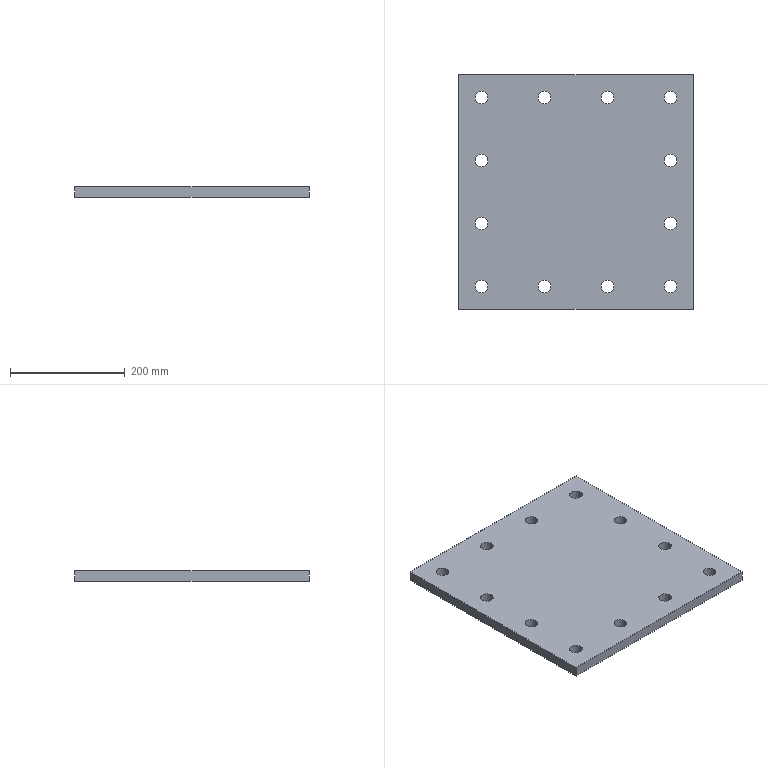Part | SolidWorks | features Extrusion 1, ICE 1 | 1 solid | 30 faces | box 410 x 410 x 18 mm | volume 2943691 mm3 | cylinder 24 | plane 6 | commonest cylinder face diameters 22 x24
STEP:
#1=CARTESIAN_POINT('',(154.,55.,0.));
#2=VERTEX_POINT('',#1);
#3=CARTESIAN_POINT('',(176.,55.,0.));
#4=VERTEX_POINT('',#3);
#5=CARTESIAN_POINT('',(165.,55.,0.));
#6=DIRECTION('',(0.,0.,1.));
#7=DIRECTION('',(1.,0.,0.));
#8=AXIS2_PLACEMENT_3D('',#5,#6,#7);
#9=CIRCLE('',#8,11.);
#10=EDGE_CURVE('',#2,#4,#9,.T.);
#11=ORIENTED_EDGE('',*,*,#10,.F.);
#12=CARTESIAN_POINT('',(154.,55.,18.));
#13=VERTEX_POINT('',#12);
#14=CARTESIAN_POINT('',(154.,55.,0.));
#15=DIRECTION('',(0.,0.,1.));
#16=VECTOR('',#15,1000.);
#17=LINE('',#14,#16);
#18=EDGE_CURVE('',#2,#13,#17,.T.);
#19=ORIENTED_EDGE('',*,*,#18,.T.);
#20=CARTESIAN_POINT('',(176.,55.,18.));
#21=VERTEX_POINT('',#20);
#22=CARTESIAN_POINT('',(165.,55.,18.));
#23=DIRECTION('',(0.,0.,1.));
#24=DIRECTION('',(1.,0.,0.));
#25=AXIS2_PLACEMENT_3D('',#22,#23,#24);
#26=CIRCLE('',#25,11.);
#27=EDGE_CURVE('',#13,#21,#26,.T.);
#28=ORIENTED_EDGE('',*,*,#27,.T.);
#29=CARTESIAN_POINT('',(176.,55.,0.));
#30=DIRECTION('',(0.,0.,1.));
#31=VECTOR('',#30,1000.);
#32=LINE('',#29,#31);
#33=EDGE_CURVE('',#4,#21,#32,.T.);
#34=ORIENTED_EDGE('',*,*,#33,.F.);
#35=EDGE_LOOP('',(#11,#19,#28,#34));
#36=FACE_OUTER_BOUND('',#35,.T.);
#37=CARTESIAN_POINT('',(165.,55.,0.));
#38=DIRECTION('',(0.,0.,1.));
#39=DIRECTION('',(1.,0.,0.));
#40=AXIS2_PLACEMENT_3D('',#37,#38,#39);
#41=CYLINDRICAL_SURFACE('',#40,11.);
#42=ADVANCED_FACE('',(#36),#41,.F.);
#43=CARTESIAN_POINT('',(44.,165.,0.));
#44=VERTEX_POINT('',#43);
#45=CARTESIAN_POINT('',(66.,165.,0.));
#46=VERTEX_POINT('',#45);
#47=CARTESIAN_POINT('',(55.,165.,0.));
#48=DIRECTION('',(0.,0.,1.));
#49=DIRECTION('',(1.,0.,0.));
#50=AXIS2_PLACEMENT_3D('',#47,#48,#49);
#51=CIRCLE('',#50,11.);
#52=EDGE_CURVE('',#44,#46,#51,.T.);
#53=ORIENTED_EDGE('',*,*,#52,.F.);
#54=CARTESIAN_POINT('',(44.,165.,18.));
#55=VERTEX_POINT('',#54);
#56=CARTESIAN_POINT('',(44.,165.,0.));
#57=DIRECTION('',(0.,0.,1.));
#58=VECTOR('',#57,1000.);
#59=LINE('',#56,#58);
#60=EDGE_CURVE('',#44,#55,#59,.T.);
#61=ORIENTED_EDGE('',*,*,#60,.T.);
#62=CARTESIAN_POINT('',(66.,165.,18.));
#63=VERTEX_POINT('',#62);
#64=CARTESIAN_POINT('',(55.,165.,18.));
#65=DIRECTION('',(0.,0.,1.));
#66=DIRECTION('',(1.,0.,0.));
#67=AXIS2_PLACEMENT_3D('',#64,#65,#66);
#68=CIRCLE('',#67,11.);
#69=EDGE_CURVE('',#55,#63,#68,.T.);
#70=ORIENTED_EDGE('',*,*,#69,.T.);
#71=CARTESIAN_POINT('',(66.,165.,0.));
#72=DIRECTION('',(0.,0.,1.));
#73=VECTOR('',#72,1000.);
#74=LINE('',#71,#73);
#75=EDGE_CURVE('',#46,#63,#74,.T.);
#76=ORIENTED_EDGE('',*,*,#75,.F.);
#77=EDGE_LOOP('',(#53,#61,#70,#76));
#78=FACE_OUTER_BOUND('',#77,.T.);
#79=CARTESIAN_POINT('',(55.,165.,0.));
#80=DIRECTION('',(0.,0.,1.));
#81=DIRECTION('',(1.,0.,0.));
#82=AXIS2_PLACEMENT_3D('',#79,#80,#81);
#83=CYLINDRICAL_SURFACE('',#82,11.);
#84=ADVANCED_FACE('',(#78),#83,.F.);
#85=CARTESIAN_POINT('',(-66.,165.,0.));
#86=VERTEX_POINT('',#85);
#87=CARTESIAN_POINT('',(-44.,165.,0.));
#88=VERTEX_POINT('',#87);
#89=CARTESIAN_POINT('',(-55.,165.,0.));
#90=DIRECTION('',(0.,0.,1.));
#91=DIRECTION('',(1.,0.,0.));
#92=AXIS2_PLACEMENT_3D('',#89,#90,#91);
#93=CIRCLE('',#92,11.);
#94=EDGE_CURVE('',#86,#88,#93,.T.);
#95=ORIENTED_EDGE('',*,*,#94,.F.);
#96=CARTESIAN_POINT('',(-66.,165.,18.));
#97=VERTEX_POINT('',#96);
#98=CARTESIAN_POINT('',(-66.,165.,0.));
#99=DIRECTION('',(0.,0.,1.));
#100=VECTOR('',#99,1000.);
#101=LINE('',#98,#100);
#102=EDGE_CURVE('',#86,#97,#101,.T.);
#103=ORIENTED_EDGE('',*,*,#102,.T.);
#104=CARTESIAN_POINT('',(-44.,165.,18.));
#105=VERTEX_POINT('',#104);
#106=CARTESIAN_POINT('',(-55.,165.,18.));
#107=DIRECTION('',(0.,0.,1.));
#108=DIRECTION('',(1.,0.,0.));
#109=AXIS2_PLACEMENT_3D('',#106,#107,#108);
#110=CIRCLE('',#109,11.);
#111=EDGE_CURVE('',#97,#105,#110,.T.);
#112=ORIENTED_EDGE('',*,*,#111,.T.);
#113=CARTESIAN_POINT('',(-44.,165.,0.));
#114=DIRECTION('',(0.,0.,1.));
#115=VECTOR('',#114,1000.);
#116=LINE('',#113,#115);
#117=EDGE_CURVE('',#88,#105,#116,.T.);
#118=ORIENTED_EDGE('',*,*,#117,.F.);
#119=EDGE_LOOP('',(#95,#103,#112,#118));
#120=FACE_OUTER_BOUND('',#119,.T.);
#121=CARTESIAN_POINT('',(-55.,165.,0.));
#122=DIRECTION('',(0.,0.,1.));
#123=DIRECTION('',(1.,0.,0.));
#124=AXIS2_PLACEMENT_3D('',#121,#122,#123);
#125=CYLINDRICAL_SURFACE('',#124,11.);
#126=ADVANCED_FACE('',(#120),#125,.F.);
#127=CARTESIAN_POINT('',(-176.,-55.,0.));
#128=VERTEX_POINT('',#127);
#129=CARTESIAN_POINT('',(-154.,-55.,0.));
#130=VERTEX_POINT('',#129);
#131=CARTESIAN_POINT('',(-165.,-55.,0.));
#132=DIRECTION('',(0.,0.,1.));
#133=DIRECTION('',(1.,0.,0.));
#134=AXIS2_PLACEMENT_3D('',#131,#132,#133);
#135=CIRCLE('',#134,11.);
#136=EDGE_CURVE('',#128,#130,#135,.T.);
#137=ORIENTED_EDGE('',*,*,#136,.F.);
#138=CARTESIAN_POINT('',(-176.,-55.,18.));
#139=VERTEX_POINT('',#138);
#140=CARTESIAN_POINT('',(-176.,-55.,0.));
#141=DIRECTION('',(0.,0.,1.));
#142=VECTOR('',#141,1000.);
#143=LINE('',#140,#142);
#144=EDGE_CURVE('',#128,#139,#143,.T.);
#145=ORIENTED_EDGE('',*,*,#144,.T.);
#146=CARTESIAN_POINT('',(-154.,-55.,18.));
#147=VERTEX_POINT('',#146);
#148=CARTESIAN_POINT('',(-165.,-55.,18.));
#149=DIRECTION('',(0.,0.,1.));
#150=DIRECTION('',(1.,0.,0.));
#151=AXIS2_PLACEMENT_3D('',#148,#149,#150);
#152=CIRCLE('',#151,11.);
#153=EDGE_CURVE('',#139,#147,#152,.T.);
#154=ORIENTED_EDGE('',*,*,#153,.T.);
#155=CARTESIAN_POINT('',(-154.,-55.,0.));
#156=DIRECTION('',(0.,0.,1.));
#157=VECTOR('',#156,1000.);
#158=LINE('',#155,#157);
#159=EDGE_CURVE('',#130,#147,#158,.T.);
#160=ORIENTED_EDGE('',*,*,#159,.F.);
#161=EDGE_LOOP('',(#137,#145,#154,#160));
#162=FACE_OUTER_BOUND('',#161,.T.);
#163=CARTESIAN_POINT('',(-165.,-55.,0.));
#164=DIRECTION('',(0.,0.,1.));
#165=DIRECTION('',(1.,0.,0.));
#166=AXIS2_PLACEMENT_3D('',#163,#164,#165);
#167=CYLINDRICAL_SURFACE('',#166,11.);
#168=ADVANCED_FACE('',(#162),#167,.F.);
#169=CARTESIAN_POINT('',(-176.,55.,0.));
#170=VERTEX_POINT('',#169);
#171=CARTESIAN_POINT('',(-154.,55.,0.));
#172=VERTEX_POINT('',#171);
#173=CARTESIAN_POINT('',(-165.,55.,0.));
#174=DIRECTION('',(0.,0.,1.));
#175=DIRECTION('',(1.,0.,0.));
#176=AXIS2_PLACEMENT_3D('',#173,#174,#175);
#177=CIRCLE('',#176,11.);
#178=EDGE_CURVE('',#170,#172,#177,.T.);
#179=ORIENTED_EDGE('',*,*,#178,.F.);
#180=CARTESIAN_POINT('',(-176.,55.,18.));
#181=VERTEX_POINT('',#180);
#182=CARTESIAN_POINT('',(-176.,55.,0.));
#183=DIRECTION('',(0.,0.,1.));
#184=VECTOR('',#183,1000.);
#185=LINE('',#182,#184);
#186=EDGE_CURVE('',#170,#181,#185,.T.);
#187=ORIENTED_EDGE('',*,*,#186,.T.);
#188=CARTESIAN_POINT('',(-154.,55.,18.));
#189=VERTEX_POINT('',#188);
#190=CARTESIAN_POINT('',(-165.,55.,18.));
#191=DIRECTION('',(0.,0.,1.));
#192=DIRECTION('',(1.,0.,0.));
#193=AXIS2_PLACEMENT_3D('',#190,#191,#192);
#194=CIRCLE('',#193,11.);
#195=EDGE_CURVE('',#181,#189,#194,.T.);
#196=ORIENTED_EDGE('',*,*,#195,.T.);
#197=CARTESIAN_POINT('',(-154.,55.,0.));
#198=DIRECTION('',(0.,0.,1.));
#199=VECTOR('',#198,1000.);
#200=LINE('',#197,#199);
#201=EDGE_CURVE('',#172,#189,#200,.T.);
#202=ORIENTED_EDGE('',*,*,#201,.F.);
#203=EDGE_LOOP('',(#179,#187,#196,#202));
#204=FACE_OUTER_BOUND('',#203,.T.);
#205=CARTESIAN_POINT('',(-165.,55.,0.));
#206=DIRECTION('',(0.,0.,1.));
#207=DIRECTION('',(1.,0.,0.));
#208=AXIS2_PLACEMENT_3D('',#205,#206,#207);
#209=CYLINDRICAL_SURFACE('',#208,11.);
#210=ADVANCED_FACE('',(#204),#209,.F.);
#211=CARTESIAN_POINT('',(-176.,-165.,0.));
#212=VERTEX_POINT('',#211);
#213=CARTESIAN_POINT('',(-154.,-165.,0.));
#214=VERTEX_POINT('',#213);
#215=CARTESIAN_POINT('',(-165.,-165.,0.));
#216=DIRECTION('',(0.,0.,1.));
#217=DIRECTION('',(1.,0.,0.));
#218=AXIS2_PLACEMENT_3D('',#215,#216,#217);
#219=CIRCLE('',#218,11.);
#220=EDGE_CURVE('',#212,#214,#219,.T.);
#221=ORIENTED_EDGE('',*,*,#220,.F.);
#222=CARTESIAN_POINT('',(-176.,-165.,18.));
#223=VERTEX_POINT('',#222);
#224=CARTESIAN_POINT('',(-176.,-165.,0.));
#225=DIRECTION('',(0.,0.,1.));
#226=VECTOR('',#225,1000.);
#227=LINE('',#224,#226);
#228=EDGE_CURVE('',#212,#223,#227,.T.);
#229=ORIENTED_EDGE('',*,*,#228,.T.);
#230=CARTESIAN_POINT('',(-154.,-165.,18.));
#231=VERTEX_POINT('',#230);
#232=CARTESIAN_POINT('',(-165.,-165.,18.));
#233=DIRECTION('',(0.,0.,1.));
#234=DIRECTION('',(1.,0.,0.));
#235=AXIS2_PLACEMENT_3D('',#232,#233,#234);
#236=CIRCLE('',#235,11.);
#237=EDGE_CURVE('',#223,#231,#236,.T.);
#238=ORIENTED_EDGE('',*,*,#237,.T.);
#239=CARTESIAN_POINT('',(-154.,-165.,0.));
#240=DIRECTION('',(0.,0.,1.));
#241=VECTOR('',#240,1000.);
#242=LINE('',#239,#241);
#243=EDGE_CURVE('',#214,#231,#242,.T.);
#244=ORIENTED_EDGE('',*,*,#243,.F.);
#245=EDGE_LOOP('',(#221,#229,#238,#244));
#246=FACE_OUTER_BOUND('',#245,.T.);
#247=CARTESIAN_POINT('',(-165.,-165.,0.));
#248=DIRECTION('',(0.,0.,1.));
#249=DIRECTION('',(1.,0.,0.));
#250=AXIS2_PLACEMENT_3D('',#247,#248,#249);
#251=CYLINDRICAL_SURFACE('',#250,11.);
#252=ADVANCED_FACE('',(#246),#251,.F.);
#253=CARTESIAN_POINT('',(154.,-165.,0.));
#254=VERTEX_POINT('',#253);
#255=CARTESIAN_POINT('',(176.,-165.,0.));
#256=VERTEX_POINT('',#255);
#257=CARTESIAN_POINT('',(165.,-165.,0.));
#258=DIRECTION('',(0.,0.,1.));
#259=DIRECTION('',(1.,0.,0.));
#260=AXIS2_PLACEMENT_3D('',#257,#258,#259);
#261=CIRCLE('',#260,11.);
#262=EDGE_CURVE('',#254,#256,#261,.T.);
#263=ORIENTED_EDGE('',*,*,#262,.F.);
#264=CARTESIAN_POINT('',(154.,-165.,18.));
#265=VERTEX_POINT('',#264);
#266=CARTESIAN_POINT('',(154.,-165.,0.));
#267=DIRECTION('',(0.,0.,1.));
#268=VECTOR('',#267,1000.);
#269=LINE('',#266,#268);
#270=EDGE_CURVE('',#254,#265,#269,.T.);
#271=ORIENTED_EDGE('',*,*,#270,.T.);
#272=CARTESIAN_POINT('',(176.,-165.,18.));
#273=VERTEX_POINT('',#272);
#274=CARTESIAN_POINT('',(165.,-165.,18.));
#275=DIRECTION('',(0.,0.,1.));
#276=DIRECTION('',(1.,0.,0.));
#277=AXIS2_PLACEMENT_3D('',#274,#275,#276);
#278=CIRCLE('',#277,11.);
#279=EDGE_CURVE('',#265,#273,#278,.T.);
#280=ORIENTED_EDGE('',*,*,#279,.T.);
#281=CARTESIAN_POINT('',(176.,-165.,0.));
#282=DIRECTION('',(0.,0.,1.));
#283=VECTOR('',#282,1000.);
#284=LINE('',#281,#283);
#285=EDGE_CURVE('',#256,#273,#284,.T.);
#286=ORIENTED_EDGE('',*,*,#285,.F.);
#287=EDGE_LOOP('',(#263,#271,#280,#286));
#288=FACE_OUTER_BOUND('',#287,.T.);
#289=CARTESIAN_POINT('',(165.,-165.,0.));
#290=DIRECTION('',(0.,0.,1.));
#291=DIRECTION('',(1.,0.,0.));
#292=AXIS2_PLACEMENT_3D('',#289,#290,#291);
#293=CYLINDRICAL_SURFACE('',#292,11.);
#294=ADVANCED_FACE('',(#288),#293,.F.);
#295=CARTESIAN_POINT('',(154.,165.,0.));
#296=VERTEX_POINT('',#295);
#297=CARTESIAN_POINT('',(176.,165.,0.));
#298=VERTEX_POINT('',#297);
#299=CARTESIAN_POINT('',(165.,165.,0.));
#300=DIRECTION('',(0.,0.,1.));
#301=DIRECTION('',(1.,0.,0.));
#302=AXIS2_PLACEMENT_3D('',#299,#300,#301);
#303=CIRCLE('',#302,11.);
#304=EDGE_CURVE('',#296,#298,#303,.T.);
#305=ORIENTED_EDGE('',*,*,#304,.F.);
#306=CARTESIAN_POINT('',(154.,165.,18.));
#307=VERTEX_POINT('',#306);
#308=CARTESIAN_POINT('',(154.,165.,0.));
#309=DIRECTION('',(0.,0.,1.));
#310=VECTOR('',#309,1000.);
#311=LINE('',#308,#310);
#312=EDGE_CURVE('',#296,#307,#311,.T.);
#313=ORIENTED_EDGE('',*,*,#312,.T.);
#314=CARTESIAN_POINT('',(176.,165.,18.));
#315=VERTEX_POINT('',#314);
#316=CARTESIAN_POINT('',(165.,165.,18.));
#317=DIRECTION('',(0.,0.,1.));
#318=DIRECTION('',(1.,0.,0.));
#319=AXIS2_PLACEMENT_3D('',#316,#317,#318);
#320=CIRCLE('',#319,11.);
#321=EDGE_CURVE('',#307,#315,#320,.T.);
#322=ORIENTED_EDGE('',*,*,#321,.T.);
#323=CARTESIAN_POINT('',(176.,165.,0.));
#324=DIRECTION('',(0.,0.,1.));
#325=VECTOR('',#324,1000.);
#326=LINE('',#323,#325);
#327=EDGE_CURVE('',#298,#315,#326,.T.);
#328=ORIENTED_EDGE('',*,*,#327,.F.);
#329=EDGE_LOOP('',(#305,#313,#322,#328));
#330=FACE_OUTER_BOUND('',#329,.T.);
#331=CARTESIAN_POINT('',(165.,165.,0.));
#332=DIRECTION('',(0.,0.,1.));
#333=DIRECTION('',(1.,0.,0.));
#334=AXIS2_PLACEMENT_3D('',#331,#332,#333);
#335=CYLINDRICAL_SURFACE('',#334,11.);
#336=ADVANCED_FACE('',(#330),#335,.F.);
#337=CARTESIAN_POINT('',(44.,-165.,0.));
#338=VERTEX_POINT('',#337);
#339=CARTESIAN_POINT('',(66.,-165.,0.));
#340=VERTEX_POINT('',#339);
#341=CARTESIAN_POINT('',(55.,-165.,0.));
#342=DIRECTION('',(0.,0.,1.));
#343=DIRECTION('',(1.,0.,0.));
#344=AXIS2_PLACEMENT_3D('',#341,#342,#343);
#345=CIRCLE('',#344,11.);
#346=EDGE_CURVE('',#338,#340,#345,.T.);
#347=ORIENTED_EDGE('',*,*,#346,.F.);
#348=CARTESIAN_POINT('',(44.,-165.,18.));
#349=VERTEX_POINT('',#348);
#350=CARTESIAN_POINT('',(44.,-165.,0.));
#351=DIRECTION('',(0.,0.,1.));
#352=VECTOR('',#351,1000.);
#353=LINE('',#350,#352);
#354=EDGE_CURVE('',#338,#349,#353,.T.);
#355=ORIENTED_EDGE('',*,*,#354,.T.);
#356=CARTESIAN_POINT('',(66.,-165.,18.));
#357=VERTEX_POINT('',#356);
#358=CARTESIAN_POINT('',(55.,-165.,18.));
#359=DIRECTION('',(0.,0.,1.));
#360=DIRECTION('',(1.,0.,0.));
#361=AXIS2_PLACEMENT_3D('',#358,#359,#360);
#362=CIRCLE('',#361,11.);
#363=EDGE_CURVE('',#349,#357,#362,.T.);
#364=ORIENTED_EDGE('',*,*,#363,.T.);
#365=CARTESIAN_POINT('',(66.,-165.,0.));
#366=DIRECTION('',(0.,0.,1.));
#367=VECTOR('',#366,1000.);
#368=LINE('',#365,#367);
#369=EDGE_CURVE('',#340,#357,#368,.T.);
#370=ORIENTED_EDGE('',*,*,#369,.F.);
#371=EDGE_LOOP('',(#347,#355,#364,#370));
#372=FACE_OUTER_BOUND('',#371,.T.);
#373=CARTESIAN_POINT('',(55.,-165.,0.));
#374=DIRECTION('',(0.,0.,1.));
#375=DIRECTION('',(1.,0.,0.));
#376=AXIS2_PLACEMENT_3D('',#373,#374,#375);
#377=CYLINDRICAL_SURFACE('',#376,11.);
#378=ADVANCED_FACE('',(#372),#377,.F.);
#379=CARTESIAN_POINT('',(-66.,-165.,0.));
#380=VERTEX_POINT('',#379);
#381=CARTESIAN_POINT('',(-44.,-165.,0.));
#382=VERTEX_POINT('',#381);
#383=CARTESIAN_POINT('',(-55.,-165.,0.));
#384=DIRECTION('',(0.,0.,1.));
#385=DIRECTION('',(1.,0.,0.));
#386=AXIS2_PLACEMENT_3D('',#383,#384,#385);
#387=CIRCLE('',#386,11.);
#388=EDGE_CURVE('',#380,#382,#387,.T.);
#389=ORIENTED_EDGE('',*,*,#388,.F.);
#390=CARTESIAN_POINT('',(-66.,-165.,18.));
#391=VERTEX_POINT('',#390);
#392=CARTESIAN_POINT('',(-66.,-165.,0.));
#393=DIRECTION('',(0.,0.,1.));
#394=VECTOR('',#393,1000.);
#395=LINE('',#392,#394);
#396=EDGE_CURVE('',#380,#391,#395,.T.);
#397=ORIENTED_EDGE('',*,*,#396,.T.);
#398=CARTESIAN_POINT('',(-44.,-165.,18.));
#399=VERTEX_POINT('',#398);
#400=CARTESIAN_POINT('',(-55.,-165.,18.));
#401=DIRECTION('',(0.,0.,1.));
#402=DIRECTION('',(1.,0.,0.));
#403=AXIS2_PLACEMENT_3D('',#400,#401,#402);
#404=CIRCLE('',#403,11.);
#405=EDGE_CURVE('',#391,#399,#404,.T.);
#406=ORIENTED_EDGE('',*,*,#405,.T.);
#407=CARTESIAN_POINT('',(-44.,-165.,0.));
#408=DIRECTION('',(0.,0.,1.));
#409=VECTOR('',#408,1000.);
#410=LINE('',#407,#409);
#411=EDGE_CURVE('',#382,#399,#410,.T.);
#412=ORIENTED_EDGE('',*,*,#411,.F.);
#413=EDGE_LOOP('',(#389,#397,#406,#412));
#414=FACE_OUTER_BOUND('',#413,.T.);
#415=CARTESIAN_POINT('',(-55.,-165.,0.));
#416=DIRECTION('',(0.,0.,1.));
#417=DIRECTION('',(1.,0.,0.));
#418=AXIS2_PLACEMENT_3D('',#415,#416,#417);
#419=CYLINDRICAL_SURFACE('',#418,11.);
#420=ADVANCED_FACE('',(#414),#419,.F.);
#421=CARTESIAN_POINT('',(154.,-55.,0.));
#422=VERTEX_POINT('',#421);
#423=CARTESIAN_POINT('',(176.,-55.,0.));
#424=VERTEX_POINT('',#423);
#425=CARTESIAN_POINT('',(165.,-55.,0.));
#426=DIRECTION('',(0.,0.,1.));
#427=DIRECTION('',(1.,0.,0.));
#428=AXIS2_PLACEMENT_3D('',#425,#426,#427);
#429=CIRCLE('',#428,11.);
#430=EDGE_CURVE('',#422,#424,#429,.T.);
#431=ORIENTED_EDGE('',*,*,#430,.F.);
#432=CARTESIAN_POINT('',(154.,-55.,18.));
#433=VERTEX_POINT('',#432);
#434=CARTESIAN_POINT('',(154.,-55.,0.));
#435=DIRECTION('',(0.,0.,1.));
#436=VECTOR('',#435,1000.);
#437=LINE('',#434,#436);
#438=EDGE_CURVE('',#422,#433,#437,.T.);
#439=ORIENTED_EDGE('',*,*,#438,.T.);
#440=CARTESIAN_POINT('',(176.,-55.,18.));
#441=VERTEX_POINT('',#440);
#442=CARTESIAN_POINT('',(165.,-55.,18.));
#443=DIRECTION('',(0.,0.,1.));
#444=DIRECTION('',(1.,0.,0.));
#445=AXIS2_PLACEMENT_3D('',#442,#443,#444);
#446=CIRCLE('',#445,11.);
#447=EDGE_CURVE('',#433,#441,#446,.T.);
#448=ORIENTED_EDGE('',*,*,#447,.T.);
#449=CARTESIAN_POINT('',(176.,-55.,0.));
#450=DIRECTION('',(0.,0.,1.));
#451=VECTOR('',#450,1000.);
#452=LINE('',#449,#451);
#453=EDGE_CURVE('',#424,#441,#452,.T.);
#454=ORIENTED_EDGE('',*,*,#453,.F.);
#455=EDGE_LOOP('',(#431,#439,#448,#454));
#456=FACE_OUTER_BOUND('',#455,.T.);
#457=CARTESIAN_POINT('',(165.,-55.,0.));
#458=DIRECTION('',(0.,0.,1.));
#459=DIRECTION('',(1.,0.,0.));
#460=AXIS2_PLACEMENT_3D('',#457,#458,#459);
#461=CYLINDRICAL_SURFACE('',#460,11.);
#462=ADVANCED_FACE('',(#456),#461,.F.);
#463=CARTESIAN_POINT('',(-176.,165.,0.));
#464=VERTEX_POINT('',#463);
#465=CARTESIAN_POINT('',(-154.,165.,0.));
#466=VERTEX_POINT('',#465);
#467=CARTESIAN_POINT('',(-165.,165.,0.));
#468=DIRECTION('',(0.,0.,1.));
#469=DIRECTION('',(1.,0.,0.));
#470=AXIS2_PLACEMENT_3D('',#467,#468,#469);
#471=CIRCLE('',#470,11.);
#472=EDGE_CURVE('',#464,#466,#471,.T.);
#473=ORIENTED_EDGE('',*,*,#472,.F.);
#474=CARTESIAN_POINT('',(-176.,165.,18.));
#475=VERTEX_POINT('',#474);
#476=CARTESIAN_POINT('',(-176.,165.,0.));
#477=DIRECTION('',(0.,0.,1.));
#478=VECTOR('',#477,1000.);
#479=LINE('',#476,#478);
#480=EDGE_CURVE('',#464,#475,#479,.T.);
#481=ORIENTED_EDGE('',*,*,#480,.T.);
#482=CARTESIAN_POINT('',(-154.,165.,18.));
#483=VERTEX_POINT('',#482);
#484=CARTESIAN_POINT('',(-165.,165.,18.));
#485=DIRECTION('',(0.,0.,1.));
#486=DIRECTION('',(1.,0.,0.));
#487=AXIS2_PLACEMENT_3D('',#484,#485,#486);
#488=CIRCLE('',#487,11.);
#489=EDGE_CURVE('',#475,#483,#488,.T.);
#490=ORIENTED_EDGE('',*,*,#489,.T.);
#491=CARTESIAN_POINT('',(-154.,165.,0.));
#492=DIRECTION('',(0.,0.,1.));
#493=VECTOR('',#492,1000.);
#494=LINE('',#491,#493);
#495=EDGE_CURVE('',#466,#483,#494,.T.);
#496=ORIENTED_EDGE('',*,*,#495,.F.);
#497=EDGE_LOOP('',(#473,#481,#490,#496));
#498=FACE_OUTER_BOUND('',#497,.T.);
#499=CARTESIAN_POINT('',(-165.,165.,0.));
#500=DIRECTION('',(0.,0.,1.));
#501=DIRECTION('',(1.,0.,0.));
#502=AXIS2_PLACEMENT_3D('',#499,#500,#501);
#503=CYLINDRICAL_SURFACE('',#502,11.);
#504=ADVANCED_FACE('',(#498),#503,.F.);
#505=CARTESIAN_POINT('',(-205.,205.,0.));
#506=VERTEX_POINT('',#505);
#507=CARTESIAN_POINT('',(-205.,-205.,0.));
#508=VERTEX_POINT('',#507);
#509=CARTESIAN_POINT('',(-205.,205.,0.));
#510=DIRECTION('',(0.,-1.,0.));
#511=VECTOR('',#510,1000.);
#512=LINE('',#509,#511);
#513=EDGE_CURVE('',#506,#508,#512,.T.);
#514=ORIENTED_EDGE('',*,*,#513,.T.);
#515=CARTESIAN_POINT('',(-205.,-205.,18.));
#516=VERTEX_POINT('',#515);
#517=CARTESIAN_POINT('',(-205.,-205.,18.));
#518=DIRECTION('',(0.,0.,-1.));
#519=VECTOR('',#518,1000.);
#520=LINE('',#517,#519);
#521=EDGE_CURVE('',#516,#508,#520,.T.);
#522=ORIENTED_EDGE('',*,*,#521,.F.);
#523=CARTESIAN_POINT('',(-205.,205.,18.));
#524=VERTEX_POINT('',#523);
#525=CARTESIAN_POINT('',(-205.,205.,18.));
#526=DIRECTION('',(0.,-1.,0.));
#527=VECTOR('',#526,1000.);
#528=LINE('',#525,#527);
#529=EDGE_CURVE('',#524,#516,#528,.T.);
#530=ORIENTED_EDGE('',*,*,#529,.F.);
#531=CARTESIAN_POINT('',(-205.,205.,18.));
#532=DIRECTION('',(0.,0.,-1.));
#533=VECTOR('',#532,1000.);
#534=LINE('',#531,#533);
#535=EDGE_CURVE('',#524,#506,#534,.T.);
#536=ORIENTED_EDGE('',*,*,#535,.T.);
#537=EDGE_LOOP('',(#514,#522,#530,#536));
#538=FACE_OUTER_BOUND('',#537,.T.);
#539=CARTESIAN_POINT('',(-205.,205.,18.));
#540=DIRECTION('',(1.,0.,0.));
#541=DIRECTION('',(0.,1.,0.));
#542=AXIS2_PLACEMENT_3D('',#539,#540,#541);
#543=PLANE('',#542);
#544=ADVANCED_FACE('',(#538),#543,.F.);
#545=CARTESIAN_POINT('',(205.,-205.,0.));
#546=VERTEX_POINT('',#545);
#547=CARTESIAN_POINT('',(205.,-205.,0.));
#548=DIRECTION('',(1.,0.,0.));
#549=VECTOR('',#548,1000.);
#550=LINE('',#547,#549);
#551=EDGE_CURVE('',#508,#546,#550,.T.);
#552=ORIENTED_EDGE('',*,*,#551,.T.);
#553=CARTESIAN_POINT('',(205.,-205.,18.));
#554=VERTEX_POINT('',#553);
#555=CARTESIAN_POINT('',(205.,-205.,18.));
#556=DIRECTION('',(0.,0.,-1.));
#557=VECTOR('',#556,1000.);
#558=LINE('',#555,#557);
#559=EDGE_CURVE('',#554,#546,#558,.T.);
#560=ORIENTED_EDGE('',*,*,#559,.F.);
#561=CARTESIAN_POINT('',(205.,-205.,18.));
#562=DIRECTION('',(1.,0.,0.));
#563=VECTOR('',#562,1000.);
#564=LINE('',#561,#563);
#565=EDGE_CURVE('',#516,#554,#564,.T.);
#566=ORIENTED_EDGE('',*,*,#565,.F.);
#567=ORIENTED_EDGE('',*,*,#521,.T.);
#568=EDGE_LOOP('',(#552,#560,#566,#567));
#569=FACE_OUTER_BOUND('',#568,.T.);
#570=CARTESIAN_POINT('',(205.,-205.,18.));
#571=DIRECTION('',(0.,1.,0.));
#572=DIRECTION('',(-1.,0.,0.));
#573=AXIS2_PLACEMENT_3D('',#570,#571,#572);
#574=PLANE('',#573);
#575=ADVANCED_FACE('',(#569),#574,.F.);
#576=CARTESIAN_POINT('',(205.,205.,0.));
#577=VERTEX_POINT('',#576);
#578=CARTESIAN_POINT('',(205.,205.,0.));
#579=DIRECTION('',(0.,1.,0.));
#580=VECTOR('',#579,1000.);
#581=LINE('',#578,#580);
#582=EDGE_CURVE('',#546,#577,#581,.T.);
#583=ORIENTED_EDGE('',*,*,#582,.T.);
#584=CARTESIAN_POINT('',(205.,205.,18.));
#585=VERTEX_POINT('',#584);
#586=CARTESIAN_POINT('',(205.,205.,18.));
#587=DIRECTION('',(0.,0.,-1.));
#588=VECTOR('',#587,1000.);
#589=LINE('',#586,#588);
#590=EDGE_CURVE('',#585,#577,#589,.T.);
#591=ORIENTED_EDGE('',*,*,#590,.F.);
#592=CARTESIAN_POINT('',(205.,205.,18.));
#593=DIRECTION('',(0.,1.,0.));
#594=VECTOR('',#593,1000.);
#595=LINE('',#592,#594);
#596=EDGE_CURVE('',#554,#585,#595,.T.);
#597=ORIENTED_EDGE('',*,*,#596,.F.);
#598=ORIENTED_EDGE('',*,*,#559,.T.);
#599=EDGE_LOOP('',(#583,#591,#597,#598));
#600=FACE_OUTER_BOUND('',#599,.T.);
#601=CARTESIAN_POINT('',(205.,205.,18.));
#602=DIRECTION('',(-1.,0.,0.));
#603=DIRECTION('',(0.,-1.,0.));
#604=AXIS2_PLACEMENT_3D('',#601,#602,#603);
#605=PLANE('',#604);
#606=ADVANCED_FACE('',(#600),#605,.F.);
#607=CARTESIAN_POINT('',(205.,205.,0.));
#608=DIRECTION('',(-1.,0.,0.));
#609=VECTOR('',#608,1000.);
#610=LINE('',#607,#609);
#611=EDGE_CURVE('',#577,#506,#610,.T.);
#612=ORIENTED_EDGE('',*,*,#611,.T.);
#613=ORIENTED_EDGE('',*,*,#535,.F.);
#614=CARTESIAN_POINT('',(205.,205.,18.));
#615=DIRECTION('',(-1.,0.,0.));
#616=VECTOR('',#615,1000.);
#617=LINE('',#614,#616);
#618=EDGE_CURVE('',#585,#524,#617,.T.);
#619=ORIENTED_EDGE('',*,*,#618,.F.);
#620=ORIENTED_EDGE('',*,*,#590,.T.);
#621=EDGE_LOOP('',(#612,#613,#619,#620));
#622=FACE_OUTER_BOUND('',#621,.T.);
#623=CARTESIAN_POINT('',(205.,205.,18.));
#624=DIRECTION('',(0.,-1.,0.));
#625=DIRECTION('',(1.,0.,0.));
#626=AXIS2_PLACEMENT_3D('',#623,#624,#625);
#627=PLANE('',#626);
#628=ADVANCED_FACE('',(#622),#627,.F.);
#629=CARTESIAN_POINT('',(165.,55.,18.));
#630=DIRECTION('',(0.,0.,1.));
#631=DIRECTION('',(1.,0.,0.));
#632=AXIS2_PLACEMENT_3D('',#629,#630,#631);
#633=CIRCLE('',#632,11.);
#634=EDGE_CURVE('',#21,#13,#633,.T.);
#635=ORIENTED_EDGE('',*,*,#634,.F.);
#636=ORIENTED_EDGE('',*,*,#27,.F.);
#637=EDGE_LOOP('',(#635,#636));
#638=FACE_BOUND('',#637,.T.);
#639=CARTESIAN_POINT('',(55.,165.,18.));
#640=DIRECTION('',(0.,0.,1.));
#641=DIRECTION('',(1.,0.,0.));
#642=AXIS2_PLACEMENT_3D('',#639,#640,#641);
#643=CIRCLE('',#642,11.);
#644=EDGE_CURVE('',#63,#55,#643,.T.);
#645=ORIENTED_EDGE('',*,*,#644,.F.);
#646=ORIENTED_EDGE('',*,*,#69,.F.);
#647=EDGE_LOOP('',(#645,#646));
#648=FACE_BOUND('',#647,.T.);
#649=CARTESIAN_POINT('',(-55.,165.,18.));
#650=DIRECTION('',(0.,0.,1.));
#651=DIRECTION('',(1.,0.,0.));
#652=AXIS2_PLACEMENT_3D('',#649,#650,#651);
#653=CIRCLE('',#652,11.);
#654=EDGE_CURVE('',#105,#97,#653,.T.);
#655=ORIENTED_EDGE('',*,*,#654,.F.);
#656=ORIENTED_EDGE('',*,*,#111,.F.);
#657=EDGE_LOOP('',(#655,#656));
#658=FACE_BOUND('',#657,.T.);
#659=CARTESIAN_POINT('',(-165.,-55.,18.));
#660=DIRECTION('',(0.,0.,1.));
#661=DIRECTION('',(1.,0.,0.));
#662=AXIS2_PLACEMENT_3D('',#659,#660,#661);
#663=CIRCLE('',#662,11.);
#664=EDGE_CURVE('',#147,#139,#663,.T.);
#665=ORIENTED_EDGE('',*,*,#664,.F.);
#666=ORIENTED_EDGE('',*,*,#153,.F.);
#667=EDGE_LOOP('',(#665,#666));
#668=FACE_BOUND('',#667,.T.);
#669=CARTESIAN_POINT('',(-165.,55.,18.));
#670=DIRECTION('',(0.,0.,1.));
#671=DIRECTION('',(1.,0.,0.));
#672=AXIS2_PLACEMENT_3D('',#669,#670,#671);
#673=CIRCLE('',#672,11.);
#674=EDGE_CURVE('',#189,#181,#673,.T.);
#675=ORIENTED_EDGE('',*,*,#674,.F.);
#676=ORIENTED_EDGE('',*,*,#195,.F.);
#677=EDGE_LOOP('',(#675,#676));
#678=FACE_BOUND('',#677,.T.);
#679=CARTESIAN_POINT('',(-165.,-165.,18.));
#680=DIRECTION('',(0.,0.,1.));
#681=DIRECTION('',(1.,0.,0.));
#682=AXIS2_PLACEMENT_3D('',#679,#680,#681);
#683=CIRCLE('',#682,11.);
#684=EDGE_CURVE('',#231,#223,#683,.T.);
#685=ORIENTED_EDGE('',*,*,#684,.F.);
#686=ORIENTED_EDGE('',*,*,#237,.F.);
#687=EDGE_LOOP('',(#685,#686));
#688=FACE_BOUND('',#687,.T.);
#689=CARTESIAN_POINT('',(165.,-165.,18.));
#690=DIRECTION('',(0.,0.,1.));
#691=DIRECTION('',(1.,0.,0.));
#692=AXIS2_PLACEMENT_3D('',#689,#690,#691);
#693=CIRCLE('',#692,11.);
#694=EDGE_CURVE('',#273,#265,#693,.T.);
#695=ORIENTED_EDGE('',*,*,#694,.F.);
#696=ORIENTED_EDGE('',*,*,#279,.F.);
#697=EDGE_LOOP('',(#695,#696));
#698=FACE_BOUND('',#697,.T.);
#699=CARTESIAN_POINT('',(165.,165.,18.));
#700=DIRECTION('',(0.,0.,1.));
#701=DIRECTION('',(1.,0.,0.));
#702=AXIS2_PLACEMENT_3D('',#699,#700,#701);
#703=CIRCLE('',#702,11.);
#704=EDGE_CURVE('',#315,#307,#703,.T.);
#705=ORIENTED_EDGE('',*,*,#704,.F.);
#706=ORIENTED_EDGE('',*,*,#321,.F.);
#707=EDGE_LOOP('',(#705,#706));
#708=FACE_BOUND('',#707,.T.);
#709=CARTESIAN_POINT('',(55.,-165.,18.));
#710=DIRECTION('',(0.,0.,1.));
#711=DIRECTION('',(1.,0.,0.));
#712=AXIS2_PLACEMENT_3D('',#709,#710,#711);
#713=CIRCLE('',#712,11.);
#714=EDGE_CURVE('',#357,#349,#713,.T.);
#715=ORIENTED_EDGE('',*,*,#714,.F.);
#716=ORIENTED_EDGE('',*,*,#363,.F.);
#717=EDGE_LOOP('',(#715,#716));
#718=FACE_BOUND('',#717,.T.);
#719=CARTESIAN_POINT('',(-55.,-165.,18.));
#720=DIRECTION('',(0.,0.,1.));
#721=DIRECTION('',(1.,0.,0.));
#722=AXIS2_PLACEMENT_3D('',#719,#720,#721);
#723=CIRCLE('',#722,11.);
#724=EDGE_CURVE('',#399,#391,#723,.T.);
#725=ORIENTED_EDGE('',*,*,#724,.F.);
#726=ORIENTED_EDGE('',*,*,#405,.F.);
#727=EDGE_LOOP('',(#725,#726));
#728=FACE_BOUND('',#727,.T.);
#729=CARTESIAN_POINT('',(165.,-55.,18.));
#730=DIRECTION('',(0.,0.,1.));
#731=DIRECTION('',(1.,0.,0.));
#732=AXIS2_PLACEMENT_3D('',#729,#730,#731);
#733=CIRCLE('',#732,11.);
#734=EDGE_CURVE('',#441,#433,#733,.T.);
#735=ORIENTED_EDGE('',*,*,#734,.F.);
#736=ORIENTED_EDGE('',*,*,#447,.F.);
#737=EDGE_LOOP('',(#735,#736));
#738=FACE_BOUND('',#737,.T.);
#739=CARTESIAN_POINT('',(-165.,165.,18.));
#740=DIRECTION('',(0.,0.,1.));
#741=DIRECTION('',(1.,0.,0.));
#742=AXIS2_PLACEMENT_3D('',#739,#740,#741);
#743=CIRCLE('',#742,11.);
#744=EDGE_CURVE('',#483,#475,#743,.T.);
#745=ORIENTED_EDGE('',*,*,#744,.F.);
#746=ORIENTED_EDGE('',*,*,#489,.F.);
#747=EDGE_LOOP('',(#745,#746));
#748=FACE_BOUND('',#747,.T.);
#749=ORIENTED_EDGE('',*,*,#529,.T.);
#750=ORIENTED_EDGE('',*,*,#565,.T.);
#751=ORIENTED_EDGE('',*,*,#596,.T.);
#752=ORIENTED_EDGE('',*,*,#618,.T.);
#753=EDGE_LOOP('',(#749,#750,#751,#752));
#754=FACE_OUTER_BOUND('',#753,.T.);
#755=CARTESIAN_POINT('',(0.,0.,18.));
#756=DIRECTION('',(0.,0.,-1.));
#757=DIRECTION('',(-1.,0.,0.));
#758=AXIS2_PLACEMENT_3D('',#755,#756,#757);
#759=PLANE('',#758);
#760=ADVANCED_FACE('',(#638,#648,#658,#668,#678,#688,#698,#708,#718,#728,#738,#748,#754),#759,.F.);
#761=CARTESIAN_POINT('',(165.,55.,0.));
#762=DIRECTION('',(0.,0.,1.));
#763=DIRECTION('',(1.,0.,0.));
#764=AXIS2_PLACEMENT_3D('',#761,#762,#763);
#765=CIRCLE('',#764,11.);
#766=EDGE_CURVE('',#4,#2,#765,.T.);
#767=ORIENTED_EDGE('',*,*,#766,.T.);
#768=ORIENTED_EDGE('',*,*,#10,.T.);
#769=EDGE_LOOP('',(#767,#768));
#770=FACE_BOUND('',#769,.T.);
#771=CARTESIAN_POINT('',(55.,165.,0.));
#772=DIRECTION('',(0.,0.,1.));
#773=DIRECTION('',(1.,0.,0.));
#774=AXIS2_PLACEMENT_3D('',#771,#772,#773);
#775=CIRCLE('',#774,11.);
#776=EDGE_CURVE('',#46,#44,#775,.T.);
#777=ORIENTED_EDGE('',*,*,#776,.T.);
#778=ORIENTED_EDGE('',*,*,#52,.T.);
#779=EDGE_LOOP('',(#777,#778));
#780=FACE_BOUND('',#779,.T.);
#781=CARTESIAN_POINT('',(-55.,165.,0.));
#782=DIRECTION('',(0.,0.,1.));
#783=DIRECTION('',(1.,0.,0.));
#784=AXIS2_PLACEMENT_3D('',#781,#782,#783);
#785=CIRCLE('',#784,11.);
#786=EDGE_CURVE('',#88,#86,#785,.T.);
#787=ORIENTED_EDGE('',*,*,#786,.T.);
#788=ORIENTED_EDGE('',*,*,#94,.T.);
#789=EDGE_LOOP('',(#787,#788));
#790=FACE_BOUND('',#789,.T.);
#791=CARTESIAN_POINT('',(-165.,-55.,0.));
#792=DIRECTION('',(0.,0.,1.));
#793=DIRECTION('',(1.,0.,0.));
#794=AXIS2_PLACEMENT_3D('',#791,#792,#793);
#795=CIRCLE('',#794,11.);
#796=EDGE_CURVE('',#130,#128,#795,.T.);
#797=ORIENTED_EDGE('',*,*,#796,.T.);
#798=ORIENTED_EDGE('',*,*,#136,.T.);
#799=EDGE_LOOP('',(#797,#798));
#800=FACE_BOUND('',#799,.T.);
#801=CARTESIAN_POINT('',(-165.,55.,0.));
#802=DIRECTION('',(0.,0.,1.));
#803=DIRECTION('',(1.,0.,0.));
#804=AXIS2_PLACEMENT_3D('',#801,#802,#803);
#805=CIRCLE('',#804,11.);
#806=EDGE_CURVE('',#172,#170,#805,.T.);
#807=ORIENTED_EDGE('',*,*,#806,.T.);
#808=ORIENTED_EDGE('',*,*,#178,.T.);
#809=EDGE_LOOP('',(#807,#808));
#810=FACE_BOUND('',#809,.T.);
#811=CARTESIAN_POINT('',(-165.,-165.,0.));
#812=DIRECTION('',(0.,0.,1.));
#813=DIRECTION('',(1.,0.,0.));
#814=AXIS2_PLACEMENT_3D('',#811,#812,#813);
#815=CIRCLE('',#814,11.);
#816=EDGE_CURVE('',#214,#212,#815,.T.);
#817=ORIENTED_EDGE('',*,*,#816,.T.);
#818=ORIENTED_EDGE('',*,*,#220,.T.);
#819=EDGE_LOOP('',(#817,#818));
#820=FACE_BOUND('',#819,.T.);
#821=CARTESIAN_POINT('',(165.,-165.,0.));
#822=DIRECTION('',(0.,0.,1.));
#823=DIRECTION('',(1.,0.,0.));
#824=AXIS2_PLACEMENT_3D('',#821,#822,#823);
#825=CIRCLE('',#824,11.);
#826=EDGE_CURVE('',#256,#254,#825,.T.);
#827=ORIENTED_EDGE('',*,*,#826,.T.);
#828=ORIENTED_EDGE('',*,*,#262,.T.);
#829=EDGE_LOOP('',(#827,#828));
#830=FACE_BOUND('',#829,.T.);
#831=CARTESIAN_POINT('',(165.,165.,0.));
#832=DIRECTION('',(0.,0.,1.));
#833=DIRECTION('',(1.,0.,0.));
#834=AXIS2_PLACEMENT_3D('',#831,#832,#833);
#835=CIRCLE('',#834,11.);
#836=EDGE_CURVE('',#298,#296,#835,.T.);
#837=ORIENTED_EDGE('',*,*,#836,.T.);
#838=ORIENTED_EDGE('',*,*,#304,.T.);
#839=EDGE_LOOP('',(#837,#838));
#840=FACE_BOUND('',#839,.T.);
#841=CARTESIAN_POINT('',(55.,-165.,0.));
#842=DIRECTION('',(0.,0.,1.));
#843=DIRECTION('',(1.,0.,0.));
#844=AXIS2_PLACEMENT_3D('',#841,#842,#843);
#845=CIRCLE('',#844,11.);
#846=EDGE_CURVE('',#340,#338,#845,.T.);
#847=ORIENTED_EDGE('',*,*,#846,.T.);
#848=ORIENTED_EDGE('',*,*,#346,.T.);
#849=EDGE_LOOP('',(#847,#848));
#850=FACE_BOUND('',#849,.T.);
#851=CARTESIAN_POINT('',(-55.,-165.,0.));
#852=DIRECTION('',(0.,0.,1.));
#853=DIRECTION('',(1.,0.,0.));
#854=AXIS2_PLACEMENT_3D('',#851,#852,#853);
#855=CIRCLE('',#854,11.);
#856=EDGE_CURVE('',#382,#380,#855,.T.);
#857=ORIENTED_EDGE('',*,*,#856,.T.);
#858=ORIENTED_EDGE('',*,*,#388,.T.);
#859=EDGE_LOOP('',(#857,#858));
#860=FACE_BOUND('',#859,.T.);
#861=CARTESIAN_POINT('',(165.,-55.,0.));
#862=DIRECTION('',(0.,0.,1.));
#863=DIRECTION('',(1.,0.,0.));
#864=AXIS2_PLACEMENT_3D('',#861,#862,#863);
#865=CIRCLE('',#864,11.);
#866=EDGE_CURVE('',#424,#422,#865,.T.);
#867=ORIENTED_EDGE('',*,*,#866,.T.);
#868=ORIENTED_EDGE('',*,*,#430,.T.);
#869=EDGE_LOOP('',(#867,#868));
#870=FACE_BOUND('',#869,.T.);
#871=CARTESIAN_POINT('',(-165.,165.,0.));
#872=DIRECTION('',(0.,0.,1.));
#873=DIRECTION('',(1.,0.,0.));
#874=AXIS2_PLACEMENT_3D('',#871,#872,#873);
#875=CIRCLE('',#874,11.);
#876=EDGE_CURVE('',#466,#464,#875,.T.);
#877=ORIENTED_EDGE('',*,*,#876,.T.);
#878=ORIENTED_EDGE('',*,*,#472,.T.);
#879=EDGE_LOOP('',(#877,#878));
#880=FACE_BOUND('',#879,.T.);
#881=ORIENTED_EDGE('',*,*,#513,.F.);
#882=ORIENTED_EDGE('',*,*,#611,.F.);
#883=ORIENTED_EDGE('',*,*,#582,.F.);
#884=ORIENTED_EDGE('',*,*,#551,.F.);
#885=EDGE_LOOP('',(#881,#882,#883,#884));
#886=FACE_OUTER_BOUND('',#885,.T.);
#887=CARTESIAN_POINT('',(0.,0.,0.));
#888=DIRECTION('',(0.,0.,-1.));
#889=DIRECTION('',(-1.,0.,0.));
#890=AXIS2_PLACEMENT_3D('',#887,#888,#889);
#891=PLANE('',#890);
#892=ADVANCED_FACE('',(#770,#780,#790,#800,#810,#820,#830,#840,#850,#860,#870,#880,#886),#891,.T.);
#893=ORIENTED_EDGE('',*,*,#480,.F.);
#894=ORIENTED_EDGE('',*,*,#876,.F.);
#895=ORIENTED_EDGE('',*,*,#495,.T.);
#896=ORIENTED_EDGE('',*,*,#744,.T.);
#897=EDGE_LOOP('',(#893,#894,#895,#896));
#898=FACE_OUTER_BOUND('',#897,.T.);
#899=CARTESIAN_POINT('',(-165.,165.,0.));
#900=DIRECTION('',(0.,0.,1.));
#901=DIRECTION('',(1.,0.,0.));
#902=AXIS2_PLACEMENT_3D('',#899,#900,#901);
#903=CYLINDRICAL_SURFACE('',#902,11.);
#904=ADVANCED_FACE('',(#898),#903,.F.);
#905=ORIENTED_EDGE('',*,*,#438,.F.);
#906=ORIENTED_EDGE('',*,*,#866,.F.);
#907=ORIENTED_EDGE('',*,*,#453,.T.);
#908=ORIENTED_EDGE('',*,*,#734,.T.);
#909=EDGE_LOOP('',(#905,#906,#907,#908));
#910=FACE_OUTER_BOUND('',#909,.T.);
#911=CARTESIAN_POINT('',(165.,-55.,0.));
#912=DIRECTION('',(0.,0.,1.));
#913=DIRECTION('',(1.,0.,0.));
#914=AXIS2_PLACEMENT_3D('',#911,#912,#913);
#915=CYLINDRICAL_SURFACE('',#914,11.);
#916=ADVANCED_FACE('',(#910),#915,.F.);
#917=ORIENTED_EDGE('',*,*,#396,.F.);
#918=ORIENTED_EDGE('',*,*,#856,.F.);
#919=ORIENTED_EDGE('',*,*,#411,.T.);
#920=ORIENTED_EDGE('',*,*,#724,.T.);
#921=EDGE_LOOP('',(#917,#918,#919,#920));
#922=FACE_OUTER_BOUND('',#921,.T.);
#923=CARTESIAN_POINT('',(-55.,-165.,0.));
#924=DIRECTION('',(0.,0.,1.));
#925=DIRECTION('',(1.,0.,0.));
#926=AXIS2_PLACEMENT_3D('',#923,#924,#925);
#927=CYLINDRICAL_SURFACE('',#926,11.);
#928=ADVANCED_FACE('',(#922),#927,.F.);
#929=ORIENTED_EDGE('',*,*,#354,.F.);
#930=ORIENTED_EDGE('',*,*,#846,.F.);
#931=ORIENTED_EDGE('',*,*,#369,.T.);
#932=ORIENTED_EDGE('',*,*,#714,.T.);
#933=EDGE_LOOP('',(#929,#930,#931,#932));
#934=FACE_OUTER_BOUND('',#933,.T.);
#935=CARTESIAN_POINT('',(55.,-165.,0.));
#936=DIRECTION('',(0.,0.,1.));
#937=DIRECTION('',(1.,0.,0.));
#938=AXIS2_PLACEMENT_3D('',#935,#936,#937);
#939=CYLINDRICAL_SURFACE('',#938,11.);
#940=ADVANCED_FACE('',(#934),#939,.F.);
#941=ORIENTED_EDGE('',*,*,#312,.F.);
#942=ORIENTED_EDGE('',*,*,#836,.F.);
#943=ORIENTED_EDGE('',*,*,#327,.T.);
#944=ORIENTED_EDGE('',*,*,#704,.T.);
#945=EDGE_LOOP('',(#941,#942,#943,#944));
#946=FACE_OUTER_BOUND('',#945,.T.);
#947=CARTESIAN_POINT('',(165.,165.,0.));
#948=DIRECTION('',(0.,0.,1.));
#949=DIRECTION('',(1.,0.,0.));
#950=AXIS2_PLACEMENT_3D('',#947,#948,#949);
#951=CYLINDRICAL_SURFACE('',#950,11.);
#952=ADVANCED_FACE('',(#946),#951,.F.);
#953=ORIENTED_EDGE('',*,*,#270,.F.);
#954=ORIENTED_EDGE('',*,*,#826,.F.);
#955=ORIENTED_EDGE('',*,*,#285,.T.);
#956=ORIENTED_EDGE('',*,*,#694,.T.);
#957=EDGE_LOOP('',(#953,#954,#955,#956));
#958=FACE_OUTER_BOUND('',#957,.T.);
#959=CARTESIAN_POINT('',(165.,-165.,0.));
#960=DIRECTION('',(0.,0.,1.));
#961=DIRECTION('',(1.,0.,0.));
#962=AXIS2_PLACEMENT_3D('',#959,#960,#961);
#963=CYLINDRICAL_SURFACE('',#962,11.);
#964=ADVANCED_FACE('',(#958),#963,.F.);
#965=ORIENTED_EDGE('',*,*,#228,.F.);
#966=ORIENTED_EDGE('',*,*,#816,.F.);
#967=ORIENTED_EDGE('',*,*,#243,.T.);
#968=ORIENTED_EDGE('',*,*,#684,.T.);
#969=EDGE_LOOP('',(#965,#966,#967,#968));
#970=FACE_OUTER_BOUND('',#969,.T.);
#971=CARTESIAN_POINT('',(-165.,-165.,0.));
#972=DIRECTION('',(0.,0.,1.));
#973=DIRECTION('',(1.,0.,0.));
#974=AXIS2_PLACEMENT_3D('',#971,#972,#973);
#975=CYLINDRICAL_SURFACE('',#974,11.);
#976=ADVANCED_FACE('',(#970),#975,.F.);
#977=ORIENTED_EDGE('',*,*,#186,.F.);
#978=ORIENTED_EDGE('',*,*,#806,.F.);
#979=ORIENTED_EDGE('',*,*,#201,.T.);
#980=ORIENTED_EDGE('',*,*,#674,.T.);
#981=EDGE_LOOP('',(#977,#978,#979,#980));
#982=FACE_OUTER_BOUND('',#981,.T.);
#983=CARTESIAN_POINT('',(-165.,55.,0.));
#984=DIRECTION('',(0.,0.,1.));
#985=DIRECTION('',(1.,0.,0.));
#986=AXIS2_PLACEMENT_3D('',#983,#984,#985);
#987=CYLINDRICAL_SURFACE('',#986,11.);
#988=ADVANCED_FACE('',(#982),#987,.F.);
#989=ORIENTED_EDGE('',*,*,#144,.F.);
#990=ORIENTED_EDGE('',*,*,#796,.F.);
#991=ORIENTED_EDGE('',*,*,#159,.T.);
#992=ORIENTED_EDGE('',*,*,#664,.T.);
#993=EDGE_LOOP('',(#989,#990,#991,#992));
#994=FACE_OUTER_BOUND('',#993,.T.);
#995=CARTESIAN_POINT('',(-165.,-55.,0.));
#996=DIRECTION('',(0.,0.,1.));
#997=DIRECTION('',(1.,0.,0.));
#998=AXIS2_PLACEMENT_3D('',#995,#996,#997);
#999=CYLINDRICAL_SURFACE('',#998,11.);
#1000=ADVANCED_FACE('',(#994),#999,.F.);
#1001=ORIENTED_EDGE('',*,*,#102,.F.);
#1002=ORIENTED_EDGE('',*,*,#786,.F.);
#1003=ORIENTED_EDGE('',*,*,#117,.T.);
#1004=ORIENTED_EDGE('',*,*,#654,.T.);
#1005=EDGE_LOOP('',(#1001,#1002,#1003,#1004));
#1006=FACE_OUTER_BOUND('',#1005,.T.);
#1007=CARTESIAN_POINT('',(-55.,165.,0.));
#1008=DIRECTION('',(0.,0.,1.));
#1009=DIRECTION('',(1.,0.,0.));
#1010=AXIS2_PLACEMENT_3D('',#1007,#1008,#1009);
#1011=CYLINDRICAL_SURFACE('',#1010,11.);
#1012=ADVANCED_FACE('',(#1006),#1011,.F.);
#1013=ORIENTED_EDGE('',*,*,#60,.F.);
#1014=ORIENTED_EDGE('',*,*,#776,.F.);
#1015=ORIENTED_EDGE('',*,*,#75,.T.);
#1016=ORIENTED_EDGE('',*,*,#644,.T.);
#1017=EDGE_LOOP('',(#1013,#1014,#1015,#1016));
#1018=FACE_OUTER_BOUND('',#1017,.T.);
#1019=CARTESIAN_POINT('',(55.,165.,0.));
#1020=DIRECTION('',(0.,0.,1.));
#1021=DIRECTION('',(1.,0.,0.));
#1022=AXIS2_PLACEMENT_3D('',#1019,#1020,#1021);
#1023=CYLINDRICAL_SURFACE('',#1022,11.);
#1024=ADVANCED_FACE('',(#1018),#1023,.F.);
#1025=ORIENTED_EDGE('',*,*,#18,.F.);
#1026=ORIENTED_EDGE('',*,*,#766,.F.);
#1027=ORIENTED_EDGE('',*,*,#33,.T.);
#1028=ORIENTED_EDGE('',*,*,#634,.T.);
#1029=EDGE_LOOP('',(#1025,#1026,#1027,#1028));
#1030=FACE_OUTER_BOUND('',#1029,.T.);
#1031=CARTESIAN_POINT('',(165.,55.,0.));
#1032=DIRECTION('',(0.,0.,1.));
#1033=DIRECTION('',(1.,0.,0.));
#1034=AXIS2_PLACEMENT_3D('',#1031,#1032,#1033);
#1035=CYLINDRICAL_SURFACE('',#1034,11.);
#1036=ADVANCED_FACE('',(#1030),#1035,.F.);
#1037=CLOSED_SHELL('',(#42,#84,#126,#168,#210,#252,#294,#336,#378,#420,#462,#504,#544,#575,#606,#628,#760,#892,#904,#916,#928,#940,#952,#964,#976,#988,#1000,#1012,#1024,#1036));
#1038=MANIFOLD_SOLID_BREP('',#1037);
#1039=CARTESIAN_POINT('',(0.,0.,0.));
#1040=DIRECTION('',(0.,0.,1.));
#1041=DIRECTION('',(1.,0.,0.));
#1042=AXIS2_PLACEMENT_3D('',#1039,#1040,#1041);
#1043=(LENGTH_UNIT()NAMED_UNIT(*)SI_UNIT(.MILLI.,.METRE.));
#1044=UNCERTAINTY_MEASURE_WITH_UNIT(LENGTH_MEASURE(0.00001),#1043,'','');
#1045=(NAMED_UNIT(*)PLANE_ANGLE_UNIT()SI_UNIT($,.RADIAN.));
#1046=(NAMED_UNIT(*)SI_UNIT($,.STERADIAN.)SOLID_ANGLE_UNIT());
#1047=(GEOMETRIC_REPRESENTATION_CONTEXT(3)GLOBAL_UNCERTAINTY_ASSIGNED_CONTEXT((#1044))GLOBAL_UNIT_ASSIGNED_CONTEXT((#1043,#1045,#1046))REPRESENTATION_CONTEXT('',''));
#1048=ADVANCED_BREP_SHAPE_REPRESENTATION('',(#1038,#1042),#1047);